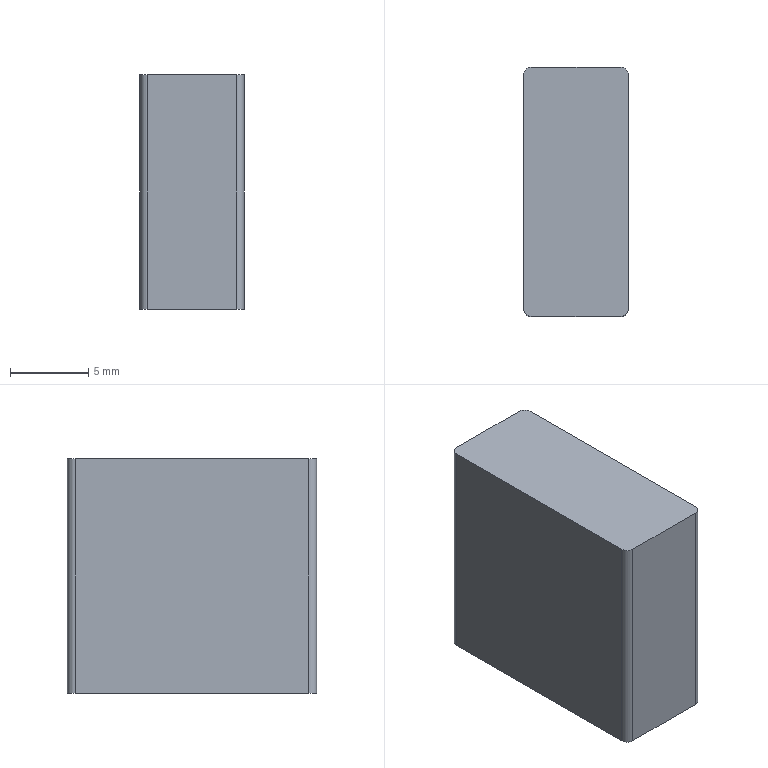Part | NX | features BREP 1 | 1 solid | 10 faces | box 6.68 x 15.946 x 15 mm | volume 1595 mm3 | plane 6 | cylinder 4 | commonest cylinder face diameters 1 x4
STEP:
#1=CARTESIAN_POINT('',(-2.84,7.973,-25.6));
#2=VERTEX_POINT('',#1);
#3=CARTESIAN_POINT('',(-3.34,7.473,-25.6));
#4=VERTEX_POINT('',#3);
#5=CARTESIAN_POINT('',(-2.84,7.473,-25.6));
#6=DIRECTION('',(0.,0.,1.));
#7=DIRECTION('',(1.,0.,0.));
#8=AXIS2_PLACEMENT_3D('',#5,#6,#7);
#9=CIRCLE('',#8,0.5);
#10=EDGE_CURVE('',#2,#4,#9,.T.);
#11=ORIENTED_EDGE('',*,*,#10,.F.);
#12=CARTESIAN_POINT('',(-2.84,7.973,-40.6));
#13=VERTEX_POINT('',#12);
#14=CARTESIAN_POINT('',(-2.84,7.973,-40.6));
#15=DIRECTION('',(0.,0.,1.));
#16=VECTOR('',#15,1000.);
#17=LINE('',#14,#16);
#18=EDGE_CURVE('',#13,#2,#17,.T.);
#19=ORIENTED_EDGE('',*,*,#18,.F.);
#20=CARTESIAN_POINT('',(-3.34,7.473,-40.6));
#21=VERTEX_POINT('',#20);
#22=CARTESIAN_POINT('',(-2.84,7.473,-40.6));
#23=DIRECTION('',(0.,0.,1.));
#24=DIRECTION('',(1.,0.,0.));
#25=AXIS2_PLACEMENT_3D('',#22,#23,#24);
#26=CIRCLE('',#25,0.5);
#27=EDGE_CURVE('',#13,#21,#26,.T.);
#28=ORIENTED_EDGE('',*,*,#27,.T.);
#29=CARTESIAN_POINT('',(-3.34,7.473,-40.6));
#30=DIRECTION('',(0.,0.,1.));
#31=VECTOR('',#30,1000.);
#32=LINE('',#29,#31);
#33=EDGE_CURVE('',#21,#4,#32,.T.);
#34=ORIENTED_EDGE('',*,*,#33,.T.);
#35=EDGE_LOOP('',(#11,#19,#28,#34));
#36=FACE_BOUND('',#35,.T.);
#37=CARTESIAN_POINT('',(-2.84,7.473,-40.6));
#38=DIRECTION('',(0.,0.,1.));
#39=DIRECTION('',(-1.,0.,0.));
#40=AXIS2_PLACEMENT_3D('',#37,#38,#39);
#41=CYLINDRICAL_SURFACE('',#40,0.5);
#42=ADVANCED_FACE('',(#36),#41,.T.);
#43=CARTESIAN_POINT('',(-3.34,-7.473,-25.6));
#44=VERTEX_POINT('',#43);
#45=CARTESIAN_POINT('',(-3.34,-7.473,-25.6));
#46=DIRECTION('',(0.,1.,0.));
#47=VECTOR('',#46,1000.);
#48=LINE('',#45,#47);
#49=EDGE_CURVE('',#44,#4,#48,.T.);
#50=ORIENTED_EDGE('',*,*,#49,.T.);
#51=ORIENTED_EDGE('',*,*,#33,.F.);
#52=CARTESIAN_POINT('',(-3.34,-7.473,-40.6));
#53=VERTEX_POINT('',#52);
#54=CARTESIAN_POINT('',(-3.34,-7.473,-40.6));
#55=DIRECTION('',(0.,1.,0.));
#56=VECTOR('',#55,1000.);
#57=LINE('',#54,#56);
#58=EDGE_CURVE('',#53,#21,#57,.T.);
#59=ORIENTED_EDGE('',*,*,#58,.F.);
#60=CARTESIAN_POINT('',(-3.34,-7.473,-40.6));
#61=DIRECTION('',(0.,0.,1.));
#62=VECTOR('',#61,1000.);
#63=LINE('',#60,#62);
#64=EDGE_CURVE('',#53,#44,#63,.T.);
#65=ORIENTED_EDGE('',*,*,#64,.T.);
#66=EDGE_LOOP('',(#50,#51,#59,#65));
#67=FACE_BOUND('',#66,.T.);
#68=CARTESIAN_POINT('',(-3.34,-7.473,-40.6));
#69=DIRECTION('',(1.,0.,0.));
#70=DIRECTION('',(0.,0.,1.));
#71=AXIS2_PLACEMENT_3D('',#68,#69,#70);
#72=PLANE('',#71);
#73=ADVANCED_FACE('',(#67),#72,.F.);
#74=CARTESIAN_POINT('',(-2.84,-7.973,-25.6));
#75=VERTEX_POINT('',#74);
#76=CARTESIAN_POINT('',(-2.84,-7.473,-25.6));
#77=DIRECTION('',(0.,0.,1.));
#78=DIRECTION('',(1.,0.,0.));
#79=AXIS2_PLACEMENT_3D('',#76,#77,#78);
#80=CIRCLE('',#79,0.5);
#81=EDGE_CURVE('',#44,#75,#80,.T.);
#82=ORIENTED_EDGE('',*,*,#81,.F.);
#83=ORIENTED_EDGE('',*,*,#64,.F.);
#84=CARTESIAN_POINT('',(-2.84,-7.973,-40.6));
#85=VERTEX_POINT('',#84);
#86=CARTESIAN_POINT('',(-2.84,-7.473,-40.6));
#87=DIRECTION('',(0.,0.,1.));
#88=DIRECTION('',(1.,0.,0.));
#89=AXIS2_PLACEMENT_3D('',#86,#87,#88);
#90=CIRCLE('',#89,0.5);
#91=EDGE_CURVE('',#53,#85,#90,.T.);
#92=ORIENTED_EDGE('',*,*,#91,.T.);
#93=CARTESIAN_POINT('',(-2.84,-7.973,-40.6));
#94=DIRECTION('',(0.,0.,1.));
#95=VECTOR('',#94,1000.);
#96=LINE('',#93,#95);
#97=EDGE_CURVE('',#85,#75,#96,.T.);
#98=ORIENTED_EDGE('',*,*,#97,.T.);
#99=EDGE_LOOP('',(#82,#83,#92,#98));
#100=FACE_BOUND('',#99,.T.);
#101=CARTESIAN_POINT('',(-2.84,-7.473,-40.6));
#102=DIRECTION('',(0.,0.,1.));
#103=DIRECTION('',(-1.,0.,0.));
#104=AXIS2_PLACEMENT_3D('',#101,#102,#103);
#105=CYLINDRICAL_SURFACE('',#104,0.5);
#106=ADVANCED_FACE('',(#100),#105,.T.);
#107=CARTESIAN_POINT('',(2.84,-7.973,-25.6));
#108=VERTEX_POINT('',#107);
#109=CARTESIAN_POINT('',(2.84,-7.973,-25.6));
#110=DIRECTION('',(-1.,0.,0.));
#111=VECTOR('',#110,1000.);
#112=LINE('',#109,#111);
#113=EDGE_CURVE('',#108,#75,#112,.T.);
#114=ORIENTED_EDGE('',*,*,#113,.T.);
#115=ORIENTED_EDGE('',*,*,#97,.F.);
#116=CARTESIAN_POINT('',(2.84,-7.973,-40.6));
#117=VERTEX_POINT('',#116);
#118=CARTESIAN_POINT('',(2.84,-7.973,-40.6));
#119=DIRECTION('',(-1.,0.,0.));
#120=VECTOR('',#119,1000.);
#121=LINE('',#118,#120);
#122=EDGE_CURVE('',#117,#85,#121,.T.);
#123=ORIENTED_EDGE('',*,*,#122,.F.);
#124=CARTESIAN_POINT('',(2.84,-7.973,-40.6));
#125=DIRECTION('',(0.,0.,1.));
#126=VECTOR('',#125,1000.);
#127=LINE('',#124,#126);
#128=EDGE_CURVE('',#117,#108,#127,.T.);
#129=ORIENTED_EDGE('',*,*,#128,.T.);
#130=EDGE_LOOP('',(#114,#115,#123,#129));
#131=FACE_BOUND('',#130,.T.);
#132=CARTESIAN_POINT('',(2.84,-7.973,-40.6));
#133=DIRECTION('',(0.,1.,0.));
#134=DIRECTION('',(0.,0.,-1.));
#135=AXIS2_PLACEMENT_3D('',#132,#133,#134);
#136=PLANE('',#135);
#137=ADVANCED_FACE('',(#131),#136,.F.);
#138=CARTESIAN_POINT('',(3.34,-7.473,-25.6));
#139=VERTEX_POINT('',#138);
#140=CARTESIAN_POINT('',(2.84,-7.473,-25.6));
#141=DIRECTION('',(0.,0.,1.));
#142=DIRECTION('',(1.,0.,0.));
#143=AXIS2_PLACEMENT_3D('',#140,#141,#142);
#144=CIRCLE('',#143,0.5);
#145=EDGE_CURVE('',#108,#139,#144,.T.);
#146=ORIENTED_EDGE('',*,*,#145,.F.);
#147=ORIENTED_EDGE('',*,*,#128,.F.);
#148=CARTESIAN_POINT('',(3.34,-7.473,-40.6));
#149=VERTEX_POINT('',#148);
#150=CARTESIAN_POINT('',(2.84,-7.473,-40.6));
#151=DIRECTION('',(0.,0.,1.));
#152=DIRECTION('',(1.,0.,0.));
#153=AXIS2_PLACEMENT_3D('',#150,#151,#152);
#154=CIRCLE('',#153,0.5);
#155=EDGE_CURVE('',#117,#149,#154,.T.);
#156=ORIENTED_EDGE('',*,*,#155,.T.);
#157=CARTESIAN_POINT('',(3.34,-7.473,-40.6));
#158=DIRECTION('',(0.,0.,1.));
#159=VECTOR('',#158,1000.);
#160=LINE('',#157,#159);
#161=EDGE_CURVE('',#149,#139,#160,.T.);
#162=ORIENTED_EDGE('',*,*,#161,.T.);
#163=EDGE_LOOP('',(#146,#147,#156,#162));
#164=FACE_BOUND('',#163,.T.);
#165=CARTESIAN_POINT('',(2.84,-7.473,-40.6));
#166=DIRECTION('',(0.,0.,1.));
#167=DIRECTION('',(-1.,0.,0.));
#168=AXIS2_PLACEMENT_3D('',#165,#166,#167);
#169=CYLINDRICAL_SURFACE('',#168,0.5);
#170=ADVANCED_FACE('',(#164),#169,.T.);
#171=CARTESIAN_POINT('',(3.34,7.473,-25.6));
#172=VERTEX_POINT('',#171);
#173=CARTESIAN_POINT('',(3.34,7.473,-25.6));
#174=DIRECTION('',(0.,-1.,0.));
#175=VECTOR('',#174,1000.);
#176=LINE('',#173,#175);
#177=EDGE_CURVE('',#172,#139,#176,.T.);
#178=ORIENTED_EDGE('',*,*,#177,.T.);
#179=ORIENTED_EDGE('',*,*,#161,.F.);
#180=CARTESIAN_POINT('',(3.34,7.473,-40.6));
#181=VERTEX_POINT('',#180);
#182=CARTESIAN_POINT('',(3.34,7.473,-40.6));
#183=DIRECTION('',(0.,-1.,0.));
#184=VECTOR('',#183,1000.);
#185=LINE('',#182,#184);
#186=EDGE_CURVE('',#181,#149,#185,.T.);
#187=ORIENTED_EDGE('',*,*,#186,.F.);
#188=CARTESIAN_POINT('',(3.34,7.473,-40.6));
#189=DIRECTION('',(0.,0.,1.));
#190=VECTOR('',#189,1000.);
#191=LINE('',#188,#190);
#192=EDGE_CURVE('',#181,#172,#191,.T.);
#193=ORIENTED_EDGE('',*,*,#192,.T.);
#194=EDGE_LOOP('',(#178,#179,#187,#193));
#195=FACE_BOUND('',#194,.T.);
#196=CARTESIAN_POINT('',(3.34,7.473,-40.6));
#197=DIRECTION('',(-1.,0.,0.));
#198=DIRECTION('',(0.,1.,0.));
#199=AXIS2_PLACEMENT_3D('',#196,#197,#198);
#200=PLANE('',#199);
#201=ADVANCED_FACE('',(#195),#200,.F.);
#202=CARTESIAN_POINT('',(2.84,7.973,-25.6));
#203=VERTEX_POINT('',#202);
#204=CARTESIAN_POINT('',(2.84,7.473,-25.6));
#205=DIRECTION('',(0.,0.,1.));
#206=DIRECTION('',(1.,0.,0.));
#207=AXIS2_PLACEMENT_3D('',#204,#205,#206);
#208=CIRCLE('',#207,0.5);
#209=EDGE_CURVE('',#172,#203,#208,.T.);
#210=ORIENTED_EDGE('',*,*,#209,.F.);
#211=ORIENTED_EDGE('',*,*,#192,.F.);
#212=CARTESIAN_POINT('',(2.84,7.973,-40.6));
#213=VERTEX_POINT('',#212);
#214=CARTESIAN_POINT('',(2.84,7.473,-40.6));
#215=DIRECTION('',(0.,0.,1.));
#216=DIRECTION('',(1.,0.,0.));
#217=AXIS2_PLACEMENT_3D('',#214,#215,#216);
#218=CIRCLE('',#217,0.5);
#219=EDGE_CURVE('',#181,#213,#218,.T.);
#220=ORIENTED_EDGE('',*,*,#219,.T.);
#221=CARTESIAN_POINT('',(2.84,7.973,-40.6));
#222=DIRECTION('',(0.,0.,1.));
#223=VECTOR('',#222,1000.);
#224=LINE('',#221,#223);
#225=EDGE_CURVE('',#213,#203,#224,.T.);
#226=ORIENTED_EDGE('',*,*,#225,.T.);
#227=EDGE_LOOP('',(#210,#211,#220,#226));
#228=FACE_BOUND('',#227,.T.);
#229=CARTESIAN_POINT('',(2.84,7.473,-40.6));
#230=DIRECTION('',(0.,0.,1.));
#231=DIRECTION('',(-1.,0.,0.));
#232=AXIS2_PLACEMENT_3D('',#229,#230,#231);
#233=CYLINDRICAL_SURFACE('',#232,0.5);
#234=ADVANCED_FACE('',(#228),#233,.T.);
#235=CARTESIAN_POINT('',(-2.84,7.973,-25.6));
#236=DIRECTION('',(1.,0.,0.));
#237=VECTOR('',#236,1000.);
#238=LINE('',#235,#237);
#239=EDGE_CURVE('',#2,#203,#238,.T.);
#240=ORIENTED_EDGE('',*,*,#239,.T.);
#241=ORIENTED_EDGE('',*,*,#225,.F.);
#242=CARTESIAN_POINT('',(-2.84,7.973,-40.6));
#243=DIRECTION('',(1.,0.,0.));
#244=VECTOR('',#243,1000.);
#245=LINE('',#242,#244);
#246=EDGE_CURVE('',#13,#213,#245,.T.);
#247=ORIENTED_EDGE('',*,*,#246,.F.);
#248=ORIENTED_EDGE('',*,*,#18,.T.);
#249=EDGE_LOOP('',(#240,#241,#247,#248));
#250=FACE_BOUND('',#249,.T.);
#251=CARTESIAN_POINT('',(-2.84,7.973,-40.6));
#252=DIRECTION('',(0.,-1.,0.));
#253=DIRECTION('',(0.,0.,1.));
#254=AXIS2_PLACEMENT_3D('',#251,#252,#253);
#255=PLANE('',#254);
#256=ADVANCED_FACE('',(#250),#255,.F.);
#257=ORIENTED_EDGE('',*,*,#27,.F.);
#258=ORIENTED_EDGE('',*,*,#246,.T.);
#259=ORIENTED_EDGE('',*,*,#219,.F.);
#260=ORIENTED_EDGE('',*,*,#186,.T.);
#261=ORIENTED_EDGE('',*,*,#155,.F.);
#262=ORIENTED_EDGE('',*,*,#122,.T.);
#263=ORIENTED_EDGE('',*,*,#91,.F.);
#264=ORIENTED_EDGE('',*,*,#58,.T.);
#265=EDGE_LOOP('',(#257,#258,#259,#260,#261,#262,#263,#264));
#266=FACE_BOUND('',#265,.T.);
#267=CARTESIAN_POINT('',(-2.84,7.473,-40.6));
#268=DIRECTION('',(0.,0.,1.));
#269=DIRECTION('',(-1.,0.,0.));
#270=AXIS2_PLACEMENT_3D('',#267,#268,#269);
#271=PLANE('',#270);
#272=ADVANCED_FACE('',(#266),#271,.F.);
#273=ORIENTED_EDGE('',*,*,#10,.T.);
#274=ORIENTED_EDGE('',*,*,#49,.F.);
#275=ORIENTED_EDGE('',*,*,#81,.T.);
#276=ORIENTED_EDGE('',*,*,#113,.F.);
#277=ORIENTED_EDGE('',*,*,#145,.T.);
#278=ORIENTED_EDGE('',*,*,#177,.F.);
#279=ORIENTED_EDGE('',*,*,#209,.T.);
#280=ORIENTED_EDGE('',*,*,#239,.F.);
#281=EDGE_LOOP('',(#273,#274,#275,#276,#277,#278,#279,#280));
#282=FACE_BOUND('',#281,.T.);
#283=CARTESIAN_POINT('',(-2.84,7.473,-25.6));
#284=DIRECTION('',(0.,0.,1.));
#285=DIRECTION('',(-1.,0.,0.));
#286=AXIS2_PLACEMENT_3D('',#283,#284,#285);
#287=PLANE('',#286);
#288=ADVANCED_FACE('',(#282),#287,.T.);
#289=CLOSED_SHELL('',(#42,#73,#106,#137,#170,#201,#234,#256,#272,#288));
#290=MANIFOLD_SOLID_BREP('',#289);
#291=(LENGTH_UNIT()NAMED_UNIT(*)SI_UNIT(.MILLI.,.METRE.));
#292=UNCERTAINTY_MEASURE_WITH_UNIT(LENGTH_MEASURE(0.00001),#291,'','');
#293=(NAMED_UNIT(*)PLANE_ANGLE_UNIT()SI_UNIT($,.RADIAN.));
#294=(NAMED_UNIT(*)SI_UNIT($,.STERADIAN.)SOLID_ANGLE_UNIT());
#295=(GEOMETRIC_REPRESENTATION_CONTEXT(3)GLOBAL_UNCERTAINTY_ASSIGNED_CONTEXT((#292))GLOBAL_UNIT_ASSIGNED_CONTEXT((#291,#293,#294))REPRESENTATION_CONTEXT('',''));
#296=ADVANCED_BREP_SHAPE_REPRESENTATION('',(#290),#295);